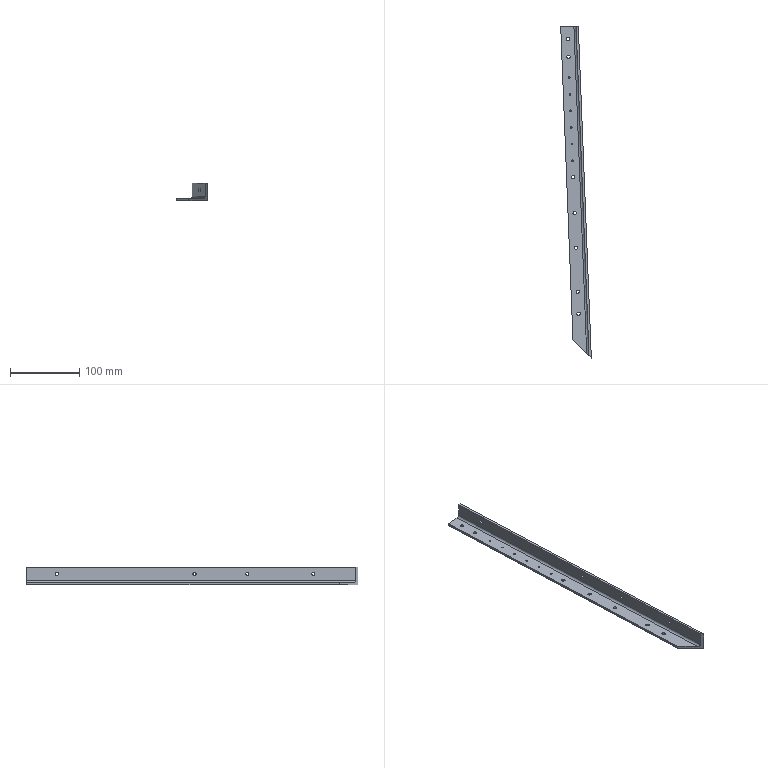Part | NX | features MG0301 nose pivot 24(right) 2 | 1 solid | 26 faces | box 44.142 x 478.899 x 25.4 mm | volume 71536 mm3 | cylinder 18 | plane 8 | commonest cylinder face diameters 4.763 x11 2.4 x6 6.35 x1
STEP:
#1=CARTESIAN_POINT('',(-10.835,-98.305,3.175));
#2=VERTEX_POINT('',#1);
#3=CARTESIAN_POINT('',(-12.034,-98.351,3.175));
#4=DIRECTION('',(0.,0.,1.));
#5=DIRECTION('',(0.9992,0.03915,0.));
#6=AXIS2_PLACEMENT_3D('',#3,#4,#5);
#7=CIRCLE('',#6,1.2);
#8=EDGE_CURVE('',#2,#2,#7,.T.);
#9=ORIENTED_EDGE('',*,*,#8,.F.);
#10=EDGE_LOOP('',(#9));
#11=FACE_BOUND('',#10,.T.);
#12=CARTESIAN_POINT('',(-8.956,-146.268,3.175));
#13=VERTEX_POINT('',#12);
#14=CARTESIAN_POINT('',(-10.155,-146.315,3.175));
#15=DIRECTION('',(0.,0.,1.));
#16=DIRECTION('',(0.9992,0.03915,0.));
#17=AXIS2_PLACEMENT_3D('',#14,#15,#16);
#18=CIRCLE('',#17,1.2);
#19=EDGE_CURVE('',#13,#13,#18,.T.);
#20=ORIENTED_EDGE('',*,*,#19,.F.);
#21=EDGE_LOOP('',(#20));
#22=FACE_BOUND('',#21,.T.);
#23=CARTESIAN_POINT('',(-7.077,-194.231,3.175));
#24=VERTEX_POINT('',#23);
#25=CARTESIAN_POINT('',(-8.276,-194.278,3.175));
#26=DIRECTION('',(0.,0.,1.));
#27=DIRECTION('',(0.9992,0.03915,0.));
#28=AXIS2_PLACEMENT_3D('',#25,#26,#27);
#29=CIRCLE('',#28,1.2);
#30=EDGE_CURVE('',#24,#24,#29,.T.);
#31=ORIENTED_EDGE('',*,*,#30,.F.);
#32=EDGE_LOOP('',(#31));
#33=FACE_BOUND('',#32,.T.);
#34=CARTESIAN_POINT('',(-2.938,-269.753,3.175));
#35=VERTEX_POINT('',#34);
#36=CARTESIAN_POINT('',(-5.319,-269.753,3.175));
#37=DIRECTION('',(0.,0.,1.));
#38=DIRECTION('',(1.,0.,0.));
#39=AXIS2_PLACEMENT_3D('',#36,#37,#38);
#40=CIRCLE('',#39,2.381);
#41=EDGE_CURVE('',#35,#35,#40,.T.);
#42=ORIENTED_EDGE('',*,*,#41,.F.);
#43=EDGE_LOOP('',(#42));
#44=FACE_BOUND('',#43,.T.);
#45=CARTESIAN_POINT('',(-0.9781,-319.782,3.175));
#46=VERTEX_POINT('',#45);
#47=CARTESIAN_POINT('',(-3.359,-319.782,3.175));
#48=DIRECTION('',(0.,0.,1.));
#49=DIRECTION('',(1.,0.,0.));
#50=AXIS2_PLACEMENT_3D('',#47,#48,#49);
#51=CIRCLE('',#50,2.381);
#52=EDGE_CURVE('',#46,#46,#51,.T.);
#53=ORIENTED_EDGE('',*,*,#52,.F.);
#54=EDGE_LOOP('',(#53));
#55=FACE_BOUND('',#54,.T.);
#56=CARTESIAN_POINT('',(2.751,-414.959,3.175));
#57=VERTEX_POINT('',#56);
#58=CARTESIAN_POINT('',(0.3693,-414.959,3.175));
#59=DIRECTION('',(0.,0.,1.));
#60=DIRECTION('',(1.,0.,0.));
#61=AXIS2_PLACEMENT_3D('',#58,#59,#60);
#62=CIRCLE('',#61,2.381);
#63=EDGE_CURVE('',#57,#57,#62,.T.);
#64=ORIENTED_EDGE('',*,*,#63,.F.);
#65=EDGE_LOOP('',(#64));
#66=FACE_BOUND('',#65,.T.);
#67=CARTESIAN_POINT('',(1.508,-383.233,3.175));
#68=VERTEX_POINT('',#67);
#69=CARTESIAN_POINT('',(-0.8735,-383.233,3.175));
#70=DIRECTION('',(0.,0.,1.));
#71=DIRECTION('',(1.,0.,0.));
#72=AXIS2_PLACEMENT_3D('',#69,#70,#71);
#73=CIRCLE('',#72,2.381);
#74=EDGE_CURVE('',#68,#68,#73,.T.);
#75=ORIENTED_EDGE('',*,*,#74,.F.);
#76=EDGE_LOOP('',(#75));
#77=FACE_BOUND('',#76,.T.);
#78=CARTESIAN_POINT('',(-12.768,-18.84,3.175));
#79=VERTEX_POINT('',#78);
#80=CARTESIAN_POINT('',(-15.149,-18.84,3.175));
#81=DIRECTION('',(0.,0.,1.));
#82=DIRECTION('',(1.,0.,0.));
#83=AXIS2_PLACEMENT_3D('',#80,#81,#82);
#84=CIRCLE('',#83,2.381);
#85=EDGE_CURVE('',#79,#79,#84,.T.);
#86=ORIENTED_EDGE('',*,*,#85,.F.);
#87=EDGE_LOOP('',(#86));
#88=FACE_BOUND('',#87,.T.);
#89=CARTESIAN_POINT('',(-11.773,-44.24,3.175));
#90=VERTEX_POINT('',#89);
#91=CARTESIAN_POINT('',(-14.154,-44.24,3.175));
#92=DIRECTION('',(0.,0.,1.));
#93=DIRECTION('',(1.,0.,0.));
#94=AXIS2_PLACEMENT_3D('',#91,#92,#93);
#95=CIRCLE('',#94,2.381);
#96=EDGE_CURVE('',#90,#90,#95,.T.);
#97=ORIENTED_EDGE('',*,*,#96,.F.);
#98=EDGE_LOOP('',(#97));
#99=FACE_BOUND('',#98,.T.);
#100=CARTESIAN_POINT('',(-4.955,-218.259,3.175));
#101=VERTEX_POINT('',#100);
#102=CARTESIAN_POINT('',(-7.337,-218.259,3.175));
#103=DIRECTION('',(0.,0.,1.));
#104=DIRECTION('',(1.,0.,0.));
#105=AXIS2_PLACEMENT_3D('',#102,#103,#104);
#106=CIRCLE('',#105,2.381);
#107=EDGE_CURVE('',#101,#101,#106,.T.);
#108=ORIENTED_EDGE('',*,*,#107,.F.);
#109=EDGE_LOOP('',(#108));
#110=FACE_BOUND('',#109,.T.);
#111=CARTESIAN_POINT('',(-6.345,-0.2486,3.175));
#112=VERTEX_POINT('',#111);
#113=CARTESIAN_POINT('',(12.142,-472.15,3.175));
#114=VERTEX_POINT('',#113);
#115=CARTESIAN_POINT('',(-6.345,-0.2486,3.175));
#116=DIRECTION('',(0.03915,-0.9992,0.));
#117=VECTOR('',#116,1000.);
#118=LINE('',#115,#117);
#119=EDGE_CURVE('',#112,#114,#118,.T.);
#120=ORIENTED_EDGE('',*,*,#119,.F.);
#121=CARTESIAN_POINT('',(-25.381,-0.9943,3.175));
#122=VERTEX_POINT('',#121);
#123=CARTESIAN_POINT('',(-6.345,-0.2486,3.175));
#124=DIRECTION('',(-0.9992,-0.03915,0.));
#125=VECTOR('',#124,1000.);
#126=LINE('',#123,#125);
#127=EDGE_CURVE('',#112,#122,#126,.T.);
#128=ORIENTED_EDGE('',*,*,#127,.T.);
#129=CARTESIAN_POINT('',(-7.716,-451.905,3.175));
#130=VERTEX_POINT('',#129);
#131=CARTESIAN_POINT('',(-25.381,-0.9943,3.175));
#132=DIRECTION('',(0.03915,-0.9992,0.));
#133=VECTOR('',#132,1000.);
#134=LINE('',#131,#133);
#135=EDGE_CURVE('',#122,#130,#134,.T.);
#136=ORIENTED_EDGE('',*,*,#135,.T.);
#137=CARTESIAN_POINT('',(-232.829,-222.393,3.175));
#138=DIRECTION('',(-0.7002,0.7139,0.));
#139=VECTOR('',#138,1000.);
#140=LINE('',#137,#139);
#141=EDGE_CURVE('',#114,#130,#140,.T.);
#142=ORIENTED_EDGE('',*,*,#141,.F.);
#143=EDGE_LOOP('',(#120,#128,#136,#142));
#144=FACE_BOUND('',#143,.T.);
#145=CARTESIAN_POINT('',(-8.017,-170.249,3.175));
#146=VERTEX_POINT('',#145);
#147=CARTESIAN_POINT('',(-9.216,-170.296,3.175));
#148=DIRECTION('',(0.,0.,1.));
#149=DIRECTION('',(0.9992,0.03915,0.));
#150=AXIS2_PLACEMENT_3D('',#147,#148,#149);
#151=CIRCLE('',#150,1.2);
#152=EDGE_CURVE('',#146,#146,#151,.T.);
#153=ORIENTED_EDGE('',*,*,#152,.F.);
#154=EDGE_LOOP('',(#153));
#155=FACE_BOUND('',#154,.T.);
#156=CARTESIAN_POINT('',(-9.896,-122.286,3.175));
#157=VERTEX_POINT('',#156);
#158=CARTESIAN_POINT('',(-11.095,-122.333,3.175));
#159=DIRECTION('',(0.,0.,1.));
#160=DIRECTION('',(0.9992,0.03915,0.));
#161=AXIS2_PLACEMENT_3D('',#158,#159,#160);
#162=CIRCLE('',#161,1.2);
#163=EDGE_CURVE('',#157,#157,#162,.T.);
#164=ORIENTED_EDGE('',*,*,#163,.F.);
#165=EDGE_LOOP('',(#164));
#166=FACE_BOUND('',#165,.T.);
#167=CARTESIAN_POINT('',(-11.775,-74.323,3.175));
#168=VERTEX_POINT('',#167);
#169=CARTESIAN_POINT('',(-12.974,-74.37,3.175));
#170=DIRECTION('',(0.,0.,1.));
#171=DIRECTION('',(0.9992,0.03915,0.));
#172=AXIS2_PLACEMENT_3D('',#169,#170,#171);
#173=CIRCLE('',#172,1.2);
#174=EDGE_CURVE('',#168,#168,#173,.T.);
#175=ORIENTED_EDGE('',*,*,#174,.F.);
#176=EDGE_LOOP('',(#175));
#177=FACE_BOUND('',#176,.T.);
#178=CARTESIAN_POINT('',(-6.345,-0.2486,3.175));
#179=DIRECTION('',(0.,0.,-1.));
#180=DIRECTION('',(1.,0.,0.));
#181=AXIS2_PLACEMENT_3D('',#178,#179,#180);
#182=PLANE('',#181);
#183=ADVANCED_FACE('',(#11,#22,#33,#44,#55,#66,#77,#88,#99,#110,#144,#155,#166,#177),#182,.F.);
#184=CARTESIAN_POINT('',(18.761,-478.899,0.));
#185=VERTEX_POINT('',#184);
#186=CARTESIAN_POINT('',(18.761,-478.899,25.4));
#187=VERTEX_POINT('',#186);
#188=CARTESIAN_POINT('',(18.761,-478.899,0.));
#189=DIRECTION('',(0.,0.,1.));
#190=VECTOR('',#189,1000.);
#191=LINE('',#188,#190);
#192=EDGE_CURVE('',#185,#187,#191,.T.);
#193=ORIENTED_EDGE('',*,*,#192,.T.);
#194=CARTESIAN_POINT('',(15.452,-475.525,25.4));
#195=VERTEX_POINT('',#194);
#196=CARTESIAN_POINT('',(-229.843,-225.438,25.4));
#197=DIRECTION('',(-0.7002,0.7139,0.));
#198=VECTOR('',#197,1000.);
#199=LINE('',#196,#198);
#200=EDGE_CURVE('',#187,#195,#199,.T.);
#201=ORIENTED_EDGE('',*,*,#200,.T.);
#202=CARTESIAN_POINT('',(15.452,-475.525,6.35));
#203=VERTEX_POINT('',#202);
#204=CARTESIAN_POINT('',(15.452,-475.525,25.4));
#205=DIRECTION('',(0.,0.,-1.));
#206=VECTOR('',#205,1000.);
#207=LINE('',#204,#206);
#208=EDGE_CURVE('',#195,#203,#207,.T.);
#209=ORIENTED_EDGE('',*,*,#208,.T.);
#210=CARTESIAN_POINT('',(12.142,-472.15,6.35));
#211=DIRECTION('',(-0.7139,-0.7002,0.));
#212=DIRECTION('',(0.7002,-0.7139,0.));
#213=AXIS2_PLACEMENT_3D('',#210,#211,#212);
#214=ELLIPSE('',#213,4.726,3.175);
#215=EDGE_CURVE('',#203,#114,#214,.F.);
#216=ORIENTED_EDGE('',*,*,#215,.T.);
#217=ORIENTED_EDGE('',*,*,#141,.T.);
#218=CARTESIAN_POINT('',(-7.716,-451.905,0.));
#219=VERTEX_POINT('',#218);
#220=CARTESIAN_POINT('',(-7.716,-451.905,0.));
#221=DIRECTION('',(0.,0.,-1.));
#222=VECTOR('',#221,1000.);
#223=LINE('',#220,#222);
#224=EDGE_CURVE('',#130,#219,#223,.T.);
#225=ORIENTED_EDGE('',*,*,#224,.T.);
#226=CARTESIAN_POINT('',(-229.843,-225.438,0.));
#227=DIRECTION('',(0.7002,-0.7139,0.));
#228=VECTOR('',#227,1000.);
#229=LINE('',#226,#228);
#230=EDGE_CURVE('',#219,#185,#229,.T.);
#231=ORIENTED_EDGE('',*,*,#230,.T.);
#232=EDGE_LOOP('',(#193,#201,#209,#216,#217,#225,#231));
#233=FACE_BOUND('',#232,.T.);
#234=CARTESIAN_POINT('',(-338.421,-114.738,-836.387));
#235=DIRECTION('',(0.7139,0.7002,0.));
#236=DIRECTION('',(-0.7002,0.7139,0.));
#237=AXIS2_PLACEMENT_3D('',#234,#235,#236);
#238=PLANE('',#237);
#239=ADVANCED_FACE('',(#233),#238,.F.);
#240=CARTESIAN_POINT('',(12.41,-316.781,15.875));
#241=VERTEX_POINT('',#240);
#242=CARTESIAN_POINT('',(12.504,-319.16,15.875));
#243=DIRECTION('',(-0.9992,-0.03915,0.));
#244=DIRECTION('',(-0.03915,0.9992,0.));
#245=AXIS2_PLACEMENT_3D('',#242,#243,#244);
#246=CIRCLE('',#245,2.381);
#247=EDGE_CURVE('',#241,#241,#246,.T.);
#248=ORIENTED_EDGE('',*,*,#247,.T.);
#249=EDGE_LOOP('',(#248));
#250=FACE_BOUND('',#249,.T.);
#251=CARTESIAN_POINT('',(16.139,-411.958,15.875));
#252=VERTEX_POINT('',#251);
#253=CARTESIAN_POINT('',(16.232,-414.337,15.875));
#254=DIRECTION('',(-0.9992,-0.03915,0.));
#255=DIRECTION('',(-0.03915,0.9992,0.));
#256=AXIS2_PLACEMENT_3D('',#253,#254,#255);
#257=CIRCLE('',#256,2.381);
#258=EDGE_CURVE('',#252,#252,#257,.T.);
#259=ORIENTED_EDGE('',*,*,#258,.T.);
#260=EDGE_LOOP('',(#259));
#261=FACE_BOUND('',#260,.T.);
#262=CARTESIAN_POINT('',(1.647,-42.037,15.875));
#263=VERTEX_POINT('',#262);
#264=CARTESIAN_POINT('',(1.74,-44.416,15.875));
#265=DIRECTION('',(-0.9992,-0.03915,0.));
#266=DIRECTION('',(-0.03915,0.9992,0.));
#267=AXIS2_PLACEMENT_3D('',#264,#265,#266);
#268=CIRCLE('',#267,2.381);
#269=EDGE_CURVE('',#263,#263,#268,.T.);
#270=ORIENTED_EDGE('',*,*,#269,.T.);
#271=EDGE_LOOP('',(#270));
#272=FACE_BOUND('',#271,.T.);
#273=CARTESIAN_POINT('',(9.427,-240.639,15.875));
#274=VERTEX_POINT('',#273);
#275=CARTESIAN_POINT('',(9.521,-243.019,15.875));
#276=DIRECTION('',(-0.9992,-0.03915,0.));
#277=DIRECTION('',(-0.03915,0.9992,0.));
#278=AXIS2_PLACEMENT_3D('',#275,#276,#277);
#279=CIRCLE('',#278,2.381);
#280=EDGE_CURVE('',#274,#274,#279,.T.);
#281=ORIENTED_EDGE('',*,*,#280,.T.);
#282=EDGE_LOOP('',(#281));
#283=FACE_BOUND('',#282,.T.);
#284=CARTESIAN_POINT('',(0.,0.,0.));
#285=VERTEX_POINT('',#284);
#286=CARTESIAN_POINT('',(0.,0.,0.));
#287=DIRECTION('',(0.03915,-0.9992,0.));
#288=VECTOR('',#287,1000.);
#289=LINE('',#286,#288);
#290=EDGE_CURVE('',#285,#185,#289,.T.);
#291=ORIENTED_EDGE('',*,*,#290,.F.);
#292=CARTESIAN_POINT('',(0.,0.,25.4));
#293=VERTEX_POINT('',#292);
#294=CARTESIAN_POINT('',(0.,0.,0.));
#295=DIRECTION('',(0.,0.,1.));
#296=VECTOR('',#295,1000.);
#297=LINE('',#294,#296);
#298=EDGE_CURVE('',#285,#293,#297,.T.);
#299=ORIENTED_EDGE('',*,*,#298,.T.);
#300=CARTESIAN_POINT('',(0.,0.,25.4));
#301=DIRECTION('',(0.03915,-0.9992,0.));
#302=VECTOR('',#301,1000.);
#303=LINE('',#300,#302);
#304=EDGE_CURVE('',#293,#187,#303,.T.);
#305=ORIENTED_EDGE('',*,*,#304,.T.);
#306=ORIENTED_EDGE('',*,*,#192,.F.);
#307=EDGE_LOOP('',(#291,#299,#305,#306));
#308=FACE_BOUND('',#307,.T.);
#309=CARTESIAN_POINT('',(0.,0.,0.));
#310=DIRECTION('',(-0.9992,-0.03915,0.));
#311=DIRECTION('',(0.03915,-0.9992,0.));
#312=AXIS2_PLACEMENT_3D('',#309,#310,#311);
#313=PLANE('',#312);
#314=ADVANCED_FACE('',(#250,#261,#272,#283,#308),#313,.F.);
#315=ORIENTED_EDGE('',*,*,#304,.F.);
#316=CARTESIAN_POINT('',(-3.173,-0.1243,25.4));
#317=VERTEX_POINT('',#316);
#318=CARTESIAN_POINT('',(0.,0.,25.4));
#319=DIRECTION('',(-0.9992,-0.03915,0.));
#320=VECTOR('',#319,1000.);
#321=LINE('',#318,#320);
#322=EDGE_CURVE('',#293,#317,#321,.T.);
#323=ORIENTED_EDGE('',*,*,#322,.T.);
#324=CARTESIAN_POINT('',(-3.173,-0.1243,25.4));
#325=DIRECTION('',(0.03915,-0.9992,0.));
#326=VECTOR('',#325,1000.);
#327=LINE('',#324,#326);
#328=EDGE_CURVE('',#317,#195,#327,.T.);
#329=ORIENTED_EDGE('',*,*,#328,.T.);
#330=ORIENTED_EDGE('',*,*,#200,.F.);
#331=EDGE_LOOP('',(#315,#323,#329,#330));
#332=FACE_BOUND('',#331,.T.);
#333=CARTESIAN_POINT('',(0.,0.,25.4));
#334=DIRECTION('',(0.,0.,-1.));
#335=DIRECTION('',(1.,0.,0.));
#336=AXIS2_PLACEMENT_3D('',#333,#334,#335);
#337=PLANE('',#336);
#338=ADVANCED_FACE('',(#332),#337,.F.);
#339=CARTESIAN_POINT('',(9.238,-316.905,15.875));
#340=VERTEX_POINT('',#339);
#341=CARTESIAN_POINT('',(9.331,-319.284,15.875));
#342=DIRECTION('',(-0.9992,-0.03915,0.));
#343=DIRECTION('',(-0.03915,0.9992,0.));
#344=AXIS2_PLACEMENT_3D('',#341,#342,#343);
#345=CIRCLE('',#344,2.381);
#346=EDGE_CURVE('',#340,#340,#345,.T.);
#347=ORIENTED_EDGE('',*,*,#346,.F.);
#348=EDGE_LOOP('',(#347));
#349=FACE_BOUND('',#348,.T.);
#350=CARTESIAN_POINT('',(12.966,-412.082,15.875));
#351=VERTEX_POINT('',#350);
#352=CARTESIAN_POINT('',(13.06,-414.461,15.875));
#353=DIRECTION('',(-0.9992,-0.03915,0.));
#354=DIRECTION('',(-0.03915,0.9992,0.));
#355=AXIS2_PLACEMENT_3D('',#352,#353,#354);
#356=CIRCLE('',#355,2.381);
#357=EDGE_CURVE('',#351,#351,#356,.T.);
#358=ORIENTED_EDGE('',*,*,#357,.F.);
#359=EDGE_LOOP('',(#358));
#360=FACE_BOUND('',#359,.T.);
#361=CARTESIAN_POINT('',(-1.526,-42.161,15.875));
#362=VERTEX_POINT('',#361);
#363=CARTESIAN_POINT('',(-1.433,-44.54,15.875));
#364=DIRECTION('',(-0.9992,-0.03915,0.));
#365=DIRECTION('',(-0.03915,0.9992,0.));
#366=AXIS2_PLACEMENT_3D('',#363,#364,#365);
#367=CIRCLE('',#366,2.381);
#368=EDGE_CURVE('',#362,#362,#367,.T.);
#369=ORIENTED_EDGE('',*,*,#368,.F.);
#370=EDGE_LOOP('',(#369));
#371=FACE_BOUND('',#370,.T.);
#372=CARTESIAN_POINT('',(6.255,-240.763,15.875));
#373=VERTEX_POINT('',#372);
#374=CARTESIAN_POINT('',(6.348,-243.143,15.875));
#375=DIRECTION('',(-0.9992,-0.03915,0.));
#376=DIRECTION('',(-0.03915,0.9992,0.));
#377=AXIS2_PLACEMENT_3D('',#374,#375,#376);
#378=CIRCLE('',#377,2.381);
#379=EDGE_CURVE('',#373,#373,#378,.T.);
#380=ORIENTED_EDGE('',*,*,#379,.F.);
#381=EDGE_LOOP('',(#380));
#382=FACE_BOUND('',#381,.T.);
#383=ORIENTED_EDGE('',*,*,#328,.F.);
#384=CARTESIAN_POINT('',(-3.173,-0.1243,6.35));
#385=VERTEX_POINT('',#384);
#386=CARTESIAN_POINT('',(-3.173,-0.1243,25.4));
#387=DIRECTION('',(0.,0.,-1.));
#388=VECTOR('',#387,1000.);
#389=LINE('',#386,#388);
#390=EDGE_CURVE('',#317,#385,#389,.T.);
#391=ORIENTED_EDGE('',*,*,#390,.T.);
#392=CARTESIAN_POINT('',(-3.173,-0.1243,6.35));
#393=DIRECTION('',(0.03915,-0.9992,0.));
#394=VECTOR('',#393,1000.);
#395=LINE('',#392,#394);
#396=EDGE_CURVE('',#385,#203,#395,.T.);
#397=ORIENTED_EDGE('',*,*,#396,.T.);
#398=ORIENTED_EDGE('',*,*,#208,.F.);
#399=EDGE_LOOP('',(#383,#391,#397,#398));
#400=FACE_BOUND('',#399,.T.);
#401=CARTESIAN_POINT('',(-3.173,-0.1243,25.4));
#402=DIRECTION('',(0.9992,0.03915,0.));
#403=DIRECTION('',(-0.03915,0.9992,0.));
#404=AXIS2_PLACEMENT_3D('',#401,#402,#403);
#405=PLANE('',#404);
#406=ADVANCED_FACE('',(#349,#360,#371,#382,#400),#405,.F.);
#407=ORIENTED_EDGE('',*,*,#396,.F.);
#408=CARTESIAN_POINT('',(-6.345,-0.2486,6.35));
#409=DIRECTION('',(-0.03915,0.9992,0.));
#410=DIRECTION('',(0.9992,0.03915,0.));
#411=AXIS2_PLACEMENT_3D('',#408,#409,#410);
#412=CIRCLE('',#411,3.175);
#413=EDGE_CURVE('',#385,#112,#412,.T.);
#414=ORIENTED_EDGE('',*,*,#413,.T.);
#415=ORIENTED_EDGE('',*,*,#119,.T.);
#416=ORIENTED_EDGE('',*,*,#215,.F.);
#417=EDGE_LOOP('',(#407,#414,#415,#416));
#418=FACE_BOUND('',#417,.T.);
#419=CARTESIAN_POINT('',(-6.345,-0.2486,6.35));
#420=DIRECTION('',(0.03915,-0.9992,0.));
#421=DIRECTION('',(0.9992,0.03915,0.));
#422=AXIS2_PLACEMENT_3D('',#419,#420,#421);
#423=CYLINDRICAL_SURFACE('',#422,3.175);
#424=ADVANCED_FACE('',(#418),#423,.F.);
#425=ORIENTED_EDGE('',*,*,#135,.F.);
#426=CARTESIAN_POINT('',(-25.381,-0.9943,0.));
#427=VERTEX_POINT('',#426);
#428=CARTESIAN_POINT('',(-25.381,-0.9943,0.));
#429=DIRECTION('',(0.,0.,-1.));
#430=VECTOR('',#429,1000.);
#431=LINE('',#428,#430);
#432=EDGE_CURVE('',#122,#427,#431,.T.);
#433=ORIENTED_EDGE('',*,*,#432,.T.);
#434=CARTESIAN_POINT('',(-25.381,-0.9943,0.));
#435=DIRECTION('',(0.03915,-0.9992,0.));
#436=VECTOR('',#435,1000.);
#437=LINE('',#434,#436);
#438=EDGE_CURVE('',#427,#219,#437,.T.);
#439=ORIENTED_EDGE('',*,*,#438,.T.);
#440=ORIENTED_EDGE('',*,*,#224,.F.);
#441=EDGE_LOOP('',(#425,#433,#439,#440));
#442=FACE_BOUND('',#441,.T.);
#443=CARTESIAN_POINT('',(-25.381,-0.9943,0.));
#444=DIRECTION('',(0.9992,0.03915,0.));
#445=DIRECTION('',(-0.03915,0.9992,0.));
#446=AXIS2_PLACEMENT_3D('',#443,#444,#445);
#447=PLANE('',#446);
#448=ADVANCED_FACE('',(#442),#447,.F.);
#449=CARTESIAN_POINT('',(-11.774,-74.37,0.));
#450=VERTEX_POINT('',#449);
#451=CARTESIAN_POINT('',(-12.974,-74.37,0.));
#452=DIRECTION('',(0.,0.,1.));
#453=DIRECTION('',(1.,0.,0.));
#454=AXIS2_PLACEMENT_3D('',#451,#452,#453);
#455=CIRCLE('',#454,1.2);
#456=EDGE_CURVE('',#450,#450,#455,.T.);
#457=ORIENTED_EDGE('',*,*,#456,.T.);
#458=EDGE_LOOP('',(#457));
#459=FACE_BOUND('',#458,.T.);
#460=CARTESIAN_POINT('',(-10.834,-98.351,0.));
#461=VERTEX_POINT('',#460);
#462=CARTESIAN_POINT('',(-12.034,-98.351,0.));
#463=DIRECTION('',(0.,0.,1.));
#464=DIRECTION('',(1.,0.,0.));
#465=AXIS2_PLACEMENT_3D('',#462,#463,#464);
#466=CIRCLE('',#465,1.2);
#467=EDGE_CURVE('',#461,#461,#466,.T.);
#468=ORIENTED_EDGE('',*,*,#467,.T.);
#469=EDGE_LOOP('',(#468));
#470=FACE_BOUND('',#469,.T.);
#471=CARTESIAN_POINT('',(-9.895,-122.333,0.));
#472=VERTEX_POINT('',#471);
#473=CARTESIAN_POINT('',(-11.095,-122.333,0.));
#474=DIRECTION('',(0.,0.,1.));
#475=DIRECTION('',(1.,0.,0.));
#476=AXIS2_PLACEMENT_3D('',#473,#474,#475);
#477=CIRCLE('',#476,1.2);
#478=EDGE_CURVE('',#472,#472,#477,.T.);
#479=ORIENTED_EDGE('',*,*,#478,.T.);
#480=EDGE_LOOP('',(#479));
#481=FACE_BOUND('',#480,.T.);
#482=CARTESIAN_POINT('',(-8.955,-146.315,0.));
#483=VERTEX_POINT('',#482);
#484=CARTESIAN_POINT('',(-10.155,-146.315,0.));
#485=DIRECTION('',(0.,0.,1.));
#486=DIRECTION('',(1.,0.,0.));
#487=AXIS2_PLACEMENT_3D('',#484,#485,#486);
#488=CIRCLE('',#487,1.2);
#489=EDGE_CURVE('',#483,#483,#488,.T.);
#490=ORIENTED_EDGE('',*,*,#489,.T.);
#491=EDGE_LOOP('',(#490));
#492=FACE_BOUND('',#491,.T.);
#493=CARTESIAN_POINT('',(-8.016,-170.296,0.));
#494=VERTEX_POINT('',#493);
#495=CARTESIAN_POINT('',(-9.216,-170.296,0.));
#496=DIRECTION('',(0.,0.,1.));
#497=DIRECTION('',(1.,0.,0.));
#498=AXIS2_PLACEMENT_3D('',#495,#496,#497);
#499=CIRCLE('',#498,1.2);
#500=EDGE_CURVE('',#494,#494,#499,.T.);
#501=ORIENTED_EDGE('',*,*,#500,.T.);
#502=EDGE_LOOP('',(#501));
#503=FACE_BOUND('',#502,.T.);
#504=CARTESIAN_POINT('',(-7.076,-194.278,0.));
#505=VERTEX_POINT('',#504);
#506=CARTESIAN_POINT('',(-8.276,-194.278,0.));
#507=DIRECTION('',(0.,0.,1.));
#508=DIRECTION('',(1.,0.,0.));
#509=AXIS2_PLACEMENT_3D('',#506,#507,#508);
#510=CIRCLE('',#509,1.2);
#511=EDGE_CURVE('',#505,#505,#510,.T.);
#512=ORIENTED_EDGE('',*,*,#511,.T.);
#513=EDGE_LOOP('',(#512));
#514=FACE_BOUND('',#513,.T.);
#515=CARTESIAN_POINT('',(-2.938,-269.753,0.));
#516=VERTEX_POINT('',#515);
#517=CARTESIAN_POINT('',(-5.319,-269.753,0.));
#518=DIRECTION('',(0.,0.,1.));
#519=DIRECTION('',(1.,0.,0.));
#520=AXIS2_PLACEMENT_3D('',#517,#518,#519);
#521=CIRCLE('',#520,2.381);
#522=EDGE_CURVE('',#516,#516,#521,.T.);
#523=ORIENTED_EDGE('',*,*,#522,.T.);
#524=EDGE_LOOP('',(#523));
#525=FACE_BOUND('',#524,.T.);
#526=CARTESIAN_POINT('',(-0.9781,-319.782,0.));
#527=VERTEX_POINT('',#526);
#528=CARTESIAN_POINT('',(-3.359,-319.782,0.));
#529=DIRECTION('',(0.,0.,1.));
#530=DIRECTION('',(1.,0.,0.));
#531=AXIS2_PLACEMENT_3D('',#528,#529,#530);
#532=CIRCLE('',#531,2.381);
#533=EDGE_CURVE('',#527,#527,#532,.T.);
#534=ORIENTED_EDGE('',*,*,#533,.T.);
#535=EDGE_LOOP('',(#534));
#536=FACE_BOUND('',#535,.T.);
#537=CARTESIAN_POINT('',(2.751,-414.959,0.));
#538=VERTEX_POINT('',#537);
#539=CARTESIAN_POINT('',(0.3693,-414.959,0.));
#540=DIRECTION('',(0.,0.,1.));
#541=DIRECTION('',(1.,0.,0.));
#542=AXIS2_PLACEMENT_3D('',#539,#540,#541);
#543=CIRCLE('',#542,2.381);
#544=EDGE_CURVE('',#538,#538,#543,.T.);
#545=ORIENTED_EDGE('',*,*,#544,.T.);
#546=EDGE_LOOP('',(#545));
#547=FACE_BOUND('',#546,.T.);
#548=CARTESIAN_POINT('',(1.508,-383.233,0.));
#549=VERTEX_POINT('',#548);
#550=CARTESIAN_POINT('',(-0.8735,-383.233,0.));
#551=DIRECTION('',(0.,0.,1.));
#552=DIRECTION('',(1.,0.,0.));
#553=AXIS2_PLACEMENT_3D('',#550,#551,#552);
#554=CIRCLE('',#553,2.381);
#555=EDGE_CURVE('',#549,#549,#554,.T.);
#556=ORIENTED_EDGE('',*,*,#555,.T.);
#557=EDGE_LOOP('',(#556));
#558=FACE_BOUND('',#557,.T.);
#559=CARTESIAN_POINT('',(-12.768,-18.84,0.));
#560=VERTEX_POINT('',#559);
#561=CARTESIAN_POINT('',(-15.149,-18.84,0.));
#562=DIRECTION('',(0.,0.,1.));
#563=DIRECTION('',(1.,0.,0.));
#564=AXIS2_PLACEMENT_3D('',#561,#562,#563);
#565=CIRCLE('',#564,2.381);
#566=EDGE_CURVE('',#560,#560,#565,.T.);
#567=ORIENTED_EDGE('',*,*,#566,.T.);
#568=EDGE_LOOP('',(#567));
#569=FACE_BOUND('',#568,.T.);
#570=CARTESIAN_POINT('',(-11.773,-44.24,0.));
#571=VERTEX_POINT('',#570);
#572=CARTESIAN_POINT('',(-14.154,-44.24,0.));
#573=DIRECTION('',(0.,0.,1.));
#574=DIRECTION('',(1.,0.,0.));
#575=AXIS2_PLACEMENT_3D('',#572,#573,#574);
#576=CIRCLE('',#575,2.381);
#577=EDGE_CURVE('',#571,#571,#576,.T.);
#578=ORIENTED_EDGE('',*,*,#577,.T.);
#579=EDGE_LOOP('',(#578));
#580=FACE_BOUND('',#579,.T.);
#581=CARTESIAN_POINT('',(-4.955,-218.259,0.));
#582=VERTEX_POINT('',#581);
#583=CARTESIAN_POINT('',(-7.337,-218.259,0.));
#584=DIRECTION('',(0.,0.,1.));
#585=DIRECTION('',(1.,0.,0.));
#586=AXIS2_PLACEMENT_3D('',#583,#584,#585);
#587=CIRCLE('',#586,2.381);
#588=EDGE_CURVE('',#582,#582,#587,.T.);
#589=ORIENTED_EDGE('',*,*,#588,.T.);
#590=EDGE_LOOP('',(#589));
#591=FACE_BOUND('',#590,.T.);
#592=ORIENTED_EDGE('',*,*,#438,.F.);
#593=CARTESIAN_POINT('',(0.,0.,0.));
#594=DIRECTION('',(0.9992,0.03915,0.));
#595=VECTOR('',#594,1000.);
#596=LINE('',#593,#595);
#597=EDGE_CURVE('',#427,#285,#596,.T.);
#598=ORIENTED_EDGE('',*,*,#597,.T.);
#599=ORIENTED_EDGE('',*,*,#290,.T.);
#600=ORIENTED_EDGE('',*,*,#230,.F.);
#601=EDGE_LOOP('',(#592,#598,#599,#600));
#602=FACE_BOUND('',#601,.T.);
#603=CARTESIAN_POINT('',(0.,0.,0.));
#604=DIRECTION('',(0.,0.,1.));
#605=DIRECTION('',(-1.,0.,0.));
#606=AXIS2_PLACEMENT_3D('',#603,#604,#605);
#607=PLANE('',#606);
#608=ADVANCED_FACE('',(#459,#470,#481,#492,#503,#514,#525,#536,#547,#558,#569,#580,#591,#602),#607,.F.);
#609=ORIENTED_EDGE('',*,*,#298,.F.);
#610=ORIENTED_EDGE('',*,*,#597,.F.);
#611=ORIENTED_EDGE('',*,*,#432,.F.);
#612=ORIENTED_EDGE('',*,*,#127,.F.);
#613=ORIENTED_EDGE('',*,*,#413,.F.);
#614=ORIENTED_EDGE('',*,*,#390,.F.);
#615=ORIENTED_EDGE('',*,*,#322,.F.);
#616=EDGE_LOOP('',(#609,#610,#611,#612,#613,#614,#615));
#617=FACE_BOUND('',#616,.T.);
#618=CARTESIAN_POINT('',(-6.345,-0.2486,6.35));
#619=DIRECTION('',(0.03915,-0.9992,0.));
#620=DIRECTION('',(0.9992,0.03915,0.));
#621=AXIS2_PLACEMENT_3D('',#618,#619,#620);
#622=PLANE('',#621);
#623=ADVANCED_FACE('',(#617),#622,.F.);
#624=ORIENTED_EDGE('',*,*,#588,.F.);
#625=EDGE_LOOP('',(#624));
#626=FACE_BOUND('',#625,.T.);
#627=ORIENTED_EDGE('',*,*,#107,.T.);
#628=EDGE_LOOP('',(#627));
#629=FACE_BOUND('',#628,.T.);
#630=CARTESIAN_POINT('',(-7.337,-218.259,63.5));
#631=DIRECTION('',(0.,0.,-1.));
#632=DIRECTION('',(1.,0.,0.));
#633=AXIS2_PLACEMENT_3D('',#630,#631,#632);
#634=CYLINDRICAL_SURFACE('',#633,2.381);
#635=ADVANCED_FACE('',(#626,#629),#634,.F.);
#636=ORIENTED_EDGE('',*,*,#577,.F.);
#637=EDGE_LOOP('',(#636));
#638=FACE_BOUND('',#637,.T.);
#639=ORIENTED_EDGE('',*,*,#96,.T.);
#640=EDGE_LOOP('',(#639));
#641=FACE_BOUND('',#640,.T.);
#642=CARTESIAN_POINT('',(-14.154,-44.24,63.5));
#643=DIRECTION('',(0.,0.,-1.));
#644=DIRECTION('',(1.,0.,0.));
#645=AXIS2_PLACEMENT_3D('',#642,#643,#644);
#646=CYLINDRICAL_SURFACE('',#645,2.381);
#647=ADVANCED_FACE('',(#638,#641),#646,.F.);
#648=ORIENTED_EDGE('',*,*,#566,.F.);
#649=EDGE_LOOP('',(#648));
#650=FACE_BOUND('',#649,.T.);
#651=ORIENTED_EDGE('',*,*,#85,.T.);
#652=EDGE_LOOP('',(#651));
#653=FACE_BOUND('',#652,.T.);
#654=CARTESIAN_POINT('',(-15.149,-18.84,63.5));
#655=DIRECTION('',(0.,0.,-1.));
#656=DIRECTION('',(1.,0.,0.));
#657=AXIS2_PLACEMENT_3D('',#654,#655,#656);
#658=CYLINDRICAL_SURFACE('',#657,2.381);
#659=ADVANCED_FACE('',(#650,#653),#658,.F.);
#660=ORIENTED_EDGE('',*,*,#555,.F.);
#661=EDGE_LOOP('',(#660));
#662=FACE_BOUND('',#661,.T.);
#663=ORIENTED_EDGE('',*,*,#74,.T.);
#664=EDGE_LOOP('',(#663));
#665=FACE_BOUND('',#664,.T.);
#666=CARTESIAN_POINT('',(-0.8735,-383.233,63.5));
#667=DIRECTION('',(0.,0.,-1.));
#668=DIRECTION('',(1.,0.,0.));
#669=AXIS2_PLACEMENT_3D('',#666,#667,#668);
#670=CYLINDRICAL_SURFACE('',#669,2.381);
#671=ADVANCED_FACE('',(#662,#665),#670,.F.);
#672=ORIENTED_EDGE('',*,*,#544,.F.);
#673=EDGE_LOOP('',(#672));
#674=FACE_BOUND('',#673,.T.);
#675=ORIENTED_EDGE('',*,*,#63,.T.);
#676=EDGE_LOOP('',(#675));
#677=FACE_BOUND('',#676,.T.);
#678=CARTESIAN_POINT('',(0.3693,-414.959,63.5));
#679=DIRECTION('',(0.,0.,-1.));
#680=DIRECTION('',(1.,0.,0.));
#681=AXIS2_PLACEMENT_3D('',#678,#679,#680);
#682=CYLINDRICAL_SURFACE('',#681,2.381);
#683=ADVANCED_FACE('',(#674,#677),#682,.F.);
#684=ORIENTED_EDGE('',*,*,#533,.F.);
#685=EDGE_LOOP('',(#684));
#686=FACE_BOUND('',#685,.T.);
#687=ORIENTED_EDGE('',*,*,#52,.T.);
#688=EDGE_LOOP('',(#687));
#689=FACE_BOUND('',#688,.T.);
#690=CARTESIAN_POINT('',(-3.359,-319.782,63.5));
#691=DIRECTION('',(0.,0.,-1.));
#692=DIRECTION('',(1.,0.,0.));
#693=AXIS2_PLACEMENT_3D('',#690,#691,#692);
#694=CYLINDRICAL_SURFACE('',#693,2.381);
#695=ADVANCED_FACE('',(#686,#689),#694,.F.);
#696=ORIENTED_EDGE('',*,*,#280,.F.);
#697=EDGE_LOOP('',(#696));
#698=FACE_BOUND('',#697,.T.);
#699=ORIENTED_EDGE('',*,*,#379,.T.);
#700=EDGE_LOOP('',(#699));
#701=FACE_BOUND('',#700,.T.);
#702=CARTESIAN_POINT('',(-15.86,-244.013,15.875));
#703=DIRECTION('',(0.9992,0.03915,0.));
#704=DIRECTION('',(-0.03915,0.9992,0.));
#705=AXIS2_PLACEMENT_3D('',#702,#703,#704);
#706=CYLINDRICAL_SURFACE('',#705,2.381);
#707=ADVANCED_FACE('',(#698,#701),#706,.F.);
#708=ORIENTED_EDGE('',*,*,#269,.F.);
#709=EDGE_LOOP('',(#708));
#710=FACE_BOUND('',#709,.T.);
#711=ORIENTED_EDGE('',*,*,#368,.T.);
#712=EDGE_LOOP('',(#711));
#713=FACE_BOUND('',#712,.T.);
#714=CARTESIAN_POINT('',(-23.64,-45.41,15.875));
#715=DIRECTION('',(0.9992,0.03915,0.));
#716=DIRECTION('',(-0.03915,0.9992,0.));
#717=AXIS2_PLACEMENT_3D('',#714,#715,#716);
#718=CYLINDRICAL_SURFACE('',#717,2.381);
#719=ADVANCED_FACE('',(#710,#713),#718,.F.);
#720=ORIENTED_EDGE('',*,*,#258,.F.);
#721=EDGE_LOOP('',(#720));
#722=FACE_BOUND('',#721,.T.);
#723=ORIENTED_EDGE('',*,*,#357,.T.);
#724=EDGE_LOOP('',(#723));
#725=FACE_BOUND('',#724,.T.);
#726=CARTESIAN_POINT('',(-9.148,-415.331,15.875));
#727=DIRECTION('',(0.9992,0.03915,0.));
#728=DIRECTION('',(-0.03915,0.9992,0.));
#729=AXIS2_PLACEMENT_3D('',#726,#727,#728);
#730=CYLINDRICAL_SURFACE('',#729,2.381);
#731=ADVANCED_FACE('',(#722,#725),#730,.F.);
#732=ORIENTED_EDGE('',*,*,#247,.F.);
#733=EDGE_LOOP('',(#732));
#734=FACE_BOUND('',#733,.T.);
#735=ORIENTED_EDGE('',*,*,#346,.T.);
#736=EDGE_LOOP('',(#735));
#737=FACE_BOUND('',#736,.T.);
#738=CARTESIAN_POINT('',(-12.877,-320.154,15.875));
#739=DIRECTION('',(0.9992,0.03915,0.));
#740=DIRECTION('',(-0.03915,0.9992,0.));
#741=AXIS2_PLACEMENT_3D('',#738,#739,#740);
#742=CYLINDRICAL_SURFACE('',#741,2.381);
#743=ADVANCED_FACE('',(#734,#737),#742,.F.);
#744=ORIENTED_EDGE('',*,*,#522,.F.);
#745=EDGE_LOOP('',(#744));
#746=FACE_BOUND('',#745,.T.);
#747=ORIENTED_EDGE('',*,*,#41,.T.);
#748=EDGE_LOOP('',(#747));
#749=FACE_BOUND('',#748,.T.);
#750=CARTESIAN_POINT('',(-5.319,-269.753,63.5));
#751=DIRECTION('',(0.,0.,-1.));
#752=DIRECTION('',(1.,0.,0.));
#753=AXIS2_PLACEMENT_3D('',#750,#751,#752);
#754=CYLINDRICAL_SURFACE('',#753,2.381);
#755=ADVANCED_FACE('',(#746,#749),#754,.F.);
#756=ORIENTED_EDGE('',*,*,#30,.T.);
#757=EDGE_LOOP('',(#756));
#758=FACE_BOUND('',#757,.T.);
#759=ORIENTED_EDGE('',*,*,#511,.F.);
#760=EDGE_LOOP('',(#759));
#761=FACE_BOUND('',#760,.T.);
#762=CARTESIAN_POINT('',(-8.276,-194.278,-6.825));
#763=DIRECTION('',(0.,0.,1.));
#764=DIRECTION('',(1.,0.,0.));
#765=AXIS2_PLACEMENT_3D('',#762,#763,#764);
#766=CYLINDRICAL_SURFACE('',#765,1.2);
#767=ADVANCED_FACE('',(#758,#761),#766,.F.);
#768=ORIENTED_EDGE('',*,*,#152,.T.);
#769=EDGE_LOOP('',(#768));
#770=FACE_BOUND('',#769,.T.);
#771=ORIENTED_EDGE('',*,*,#500,.F.);
#772=EDGE_LOOP('',(#771));
#773=FACE_BOUND('',#772,.T.);
#774=CARTESIAN_POINT('',(-9.216,-170.296,-6.825));
#775=DIRECTION('',(0.,0.,1.));
#776=DIRECTION('',(1.,0.,0.));
#777=AXIS2_PLACEMENT_3D('',#774,#775,#776);
#778=CYLINDRICAL_SURFACE('',#777,1.2);
#779=ADVANCED_FACE('',(#770,#773),#778,.F.);
#780=ORIENTED_EDGE('',*,*,#19,.T.);
#781=EDGE_LOOP('',(#780));
#782=FACE_BOUND('',#781,.T.);
#783=ORIENTED_EDGE('',*,*,#489,.F.);
#784=EDGE_LOOP('',(#783));
#785=FACE_BOUND('',#784,.T.);
#786=CARTESIAN_POINT('',(-10.155,-146.315,-6.825));
#787=DIRECTION('',(0.,0.,1.));
#788=DIRECTION('',(1.,0.,0.));
#789=AXIS2_PLACEMENT_3D('',#786,#787,#788);
#790=CYLINDRICAL_SURFACE('',#789,1.2);
#791=ADVANCED_FACE('',(#782,#785),#790,.F.);
#792=ORIENTED_EDGE('',*,*,#163,.T.);
#793=EDGE_LOOP('',(#792));
#794=FACE_BOUND('',#793,.T.);
#795=ORIENTED_EDGE('',*,*,#478,.F.);
#796=EDGE_LOOP('',(#795));
#797=FACE_BOUND('',#796,.T.);
#798=CARTESIAN_POINT('',(-11.095,-122.333,-6.825));
#799=DIRECTION('',(0.,0.,1.));
#800=DIRECTION('',(1.,0.,0.));
#801=AXIS2_PLACEMENT_3D('',#798,#799,#800);
#802=CYLINDRICAL_SURFACE('',#801,1.2);
#803=ADVANCED_FACE('',(#794,#797),#802,.F.);
#804=ORIENTED_EDGE('',*,*,#8,.T.);
#805=EDGE_LOOP('',(#804));
#806=FACE_BOUND('',#805,.T.);
#807=ORIENTED_EDGE('',*,*,#467,.F.);
#808=EDGE_LOOP('',(#807));
#809=FACE_BOUND('',#808,.T.);
#810=CARTESIAN_POINT('',(-12.034,-98.351,-6.825));
#811=DIRECTION('',(0.,0.,1.));
#812=DIRECTION('',(1.,0.,0.));
#813=AXIS2_PLACEMENT_3D('',#810,#811,#812);
#814=CYLINDRICAL_SURFACE('',#813,1.2);
#815=ADVANCED_FACE('',(#806,#809),#814,.F.);
#816=ORIENTED_EDGE('',*,*,#174,.T.);
#817=EDGE_LOOP('',(#816));
#818=FACE_BOUND('',#817,.T.);
#819=ORIENTED_EDGE('',*,*,#456,.F.);
#820=EDGE_LOOP('',(#819));
#821=FACE_BOUND('',#820,.T.);
#822=CARTESIAN_POINT('',(-12.974,-74.37,-6.825));
#823=DIRECTION('',(0.,0.,1.));
#824=DIRECTION('',(1.,0.,0.));
#825=AXIS2_PLACEMENT_3D('',#822,#823,#824);
#826=CYLINDRICAL_SURFACE('',#825,1.2);
#827=ADVANCED_FACE('',(#818,#821),#826,.F.);
#828=CLOSED_SHELL('',(#183,#239,#314,#338,#406,#424,#448,#608,#623,#635,#647,#659,#671,#683,#695,#707,#719,#731,#743,#755,#767,#779,#791,#803,#815,#827));
#829=MANIFOLD_SOLID_BREP('',#828);
#830=(LENGTH_UNIT()NAMED_UNIT(*)SI_UNIT(.MILLI.,.METRE.));
#831=UNCERTAINTY_MEASURE_WITH_UNIT(LENGTH_MEASURE(0.00001),#830,'','');
#832=(NAMED_UNIT(*)PLANE_ANGLE_UNIT()SI_UNIT($,.RADIAN.));
#833=(NAMED_UNIT(*)SI_UNIT($,.STERADIAN.)SOLID_ANGLE_UNIT());
#834=(GEOMETRIC_REPRESENTATION_CONTEXT(3)GLOBAL_UNCERTAINTY_ASSIGNED_CONTEXT((#831))GLOBAL_UNIT_ASSIGNED_CONTEXT((#830,#832,#833))REPRESENTATION_CONTEXT('',''));
#835=ADVANCED_BREP_SHAPE_REPRESENTATION('',(#829),#834);